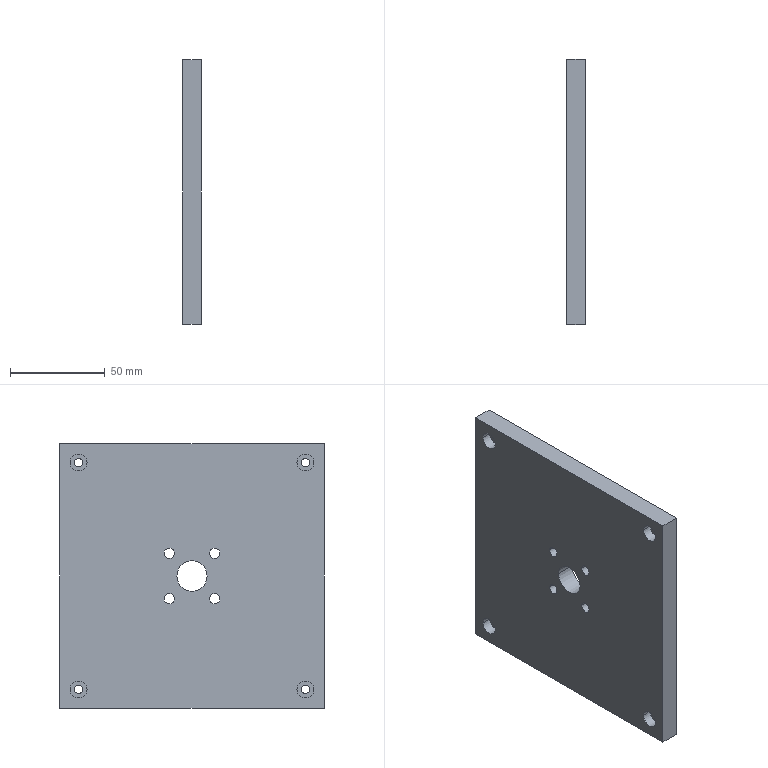Part | STEP file | 04-06 Suction cylinder fixing plate | 1 solid | 36 faces | box 10 x 140 x 140 mm | volume 191449 mm3 | cylinder 26 | plane 10 | commonest cylinder face diameters 4.5 x8 5.5 x8 9 x8 16 x2